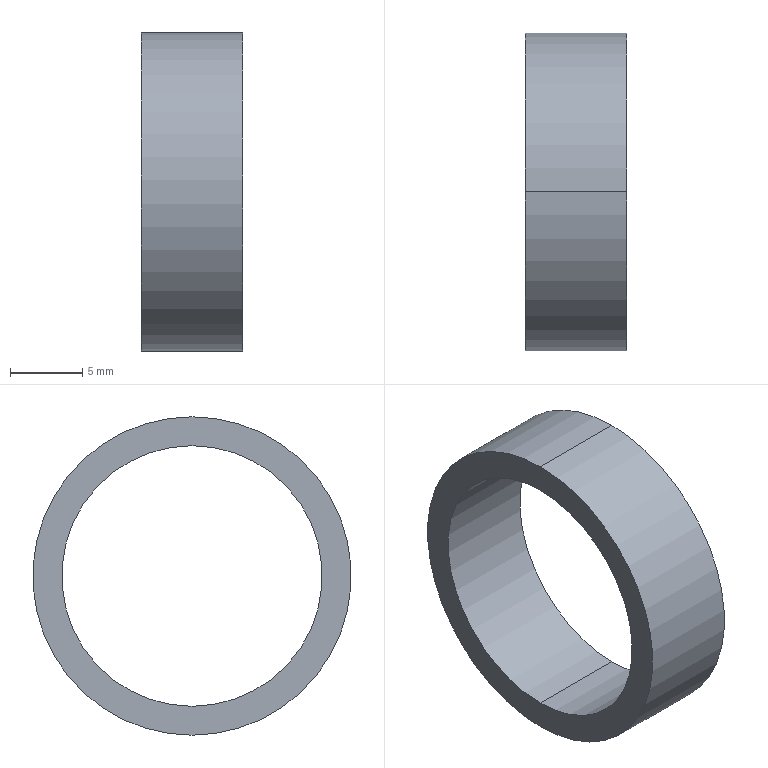Part | SolidWorks | features BaseBody 1 | 1 solid | 6 faces | box 7 x 22 x 22 mm | volume 879.646 mm3 | cylinder 4 | plane 2 | commonest cylinder face diameters 18 x2 22 x2
STEP:
#1=CARTESIAN_POINT('',(-3.5,0.,-11.));
#2=VERTEX_POINT('',#1);
#3=CARTESIAN_POINT('',(-3.5,0.,11.));
#4=VERTEX_POINT('',#3);
#5=CARTESIAN_POINT('',(-3.5,0.,0.));
#6=DIRECTION('',(1.,0.,0.));
#7=DIRECTION('',(0.,0.,-1.));
#8=AXIS2_PLACEMENT_3D('',#5,#6,#7);
#9=CIRCLE('',#8,11.);
#10=EDGE_CURVE('',#2,#4,#9,.T.);
#11=ORIENTED_EDGE('',*,*,#10,.T.);
#12=CARTESIAN_POINT('',(3.5,0.,11.));
#13=VERTEX_POINT('',#12);
#14=CARTESIAN_POINT('',(-3.5,0.,11.));
#15=DIRECTION('',(1.,0.,0.));
#16=VECTOR('',#15,1000.);
#17=LINE('',#14,#16);
#18=EDGE_CURVE('',#4,#13,#17,.T.);
#19=ORIENTED_EDGE('',*,*,#18,.T.);
#20=CARTESIAN_POINT('',(3.5,0.,-11.));
#21=VERTEX_POINT('',#20);
#22=CARTESIAN_POINT('',(3.5,0.,0.));
#23=DIRECTION('',(-1.,0.,0.));
#24=DIRECTION('',(0.,0.,-1.));
#25=AXIS2_PLACEMENT_3D('',#22,#23,#24);
#26=CIRCLE('',#25,11.);
#27=EDGE_CURVE('',#13,#21,#26,.T.);
#28=ORIENTED_EDGE('',*,*,#27,.T.);
#29=CARTESIAN_POINT('',(-3.5,0.,-11.));
#30=DIRECTION('',(1.,0.,0.));
#31=VECTOR('',#30,1000.);
#32=LINE('',#29,#31);
#33=EDGE_CURVE('',#2,#21,#32,.T.);
#34=ORIENTED_EDGE('',*,*,#33,.F.);
#35=EDGE_LOOP('',(#11,#19,#28,#34));
#36=FACE_OUTER_BOUND('',#35,.T.);
#37=CARTESIAN_POINT('',(-3.5,0.,0.));
#38=DIRECTION('',(1.,0.,0.));
#39=DIRECTION('',(0.,0.,-1.));
#40=AXIS2_PLACEMENT_3D('',#37,#38,#39);
#41=CYLINDRICAL_SURFACE('',#40,11.);
#42=ADVANCED_FACE('',(#36),#41,.T.);
#43=CARTESIAN_POINT('',(-3.5,0.,-9.));
#44=VERTEX_POINT('',#43);
#45=CARTESIAN_POINT('',(-3.5,0.,9.));
#46=VERTEX_POINT('',#45);
#47=CARTESIAN_POINT('',(-3.5,0.,0.));
#48=DIRECTION('',(-1.,0.,0.));
#49=DIRECTION('',(0.,0.,-1.));
#50=AXIS2_PLACEMENT_3D('',#47,#48,#49);
#51=CIRCLE('',#50,9.);
#52=EDGE_CURVE('',#44,#46,#51,.T.);
#53=ORIENTED_EDGE('',*,*,#52,.T.);
#54=CARTESIAN_POINT('',(3.5,0.,9.));
#55=VERTEX_POINT('',#54);
#56=CARTESIAN_POINT('',(-4.5,0.,9.));
#57=DIRECTION('',(1.,0.,0.));
#58=VECTOR('',#57,1000.);
#59=LINE('',#56,#58);
#60=EDGE_CURVE('',#46,#55,#59,.T.);
#61=ORIENTED_EDGE('',*,*,#60,.T.);
#62=CARTESIAN_POINT('',(3.5,0.,-9.));
#63=VERTEX_POINT('',#62);
#64=CARTESIAN_POINT('',(3.5,0.,0.));
#65=DIRECTION('',(-1.,0.,0.));
#66=DIRECTION('',(0.,0.,-1.));
#67=AXIS2_PLACEMENT_3D('',#64,#65,#66);
#68=CIRCLE('',#67,9.);
#69=EDGE_CURVE('',#63,#55,#68,.T.);
#70=ORIENTED_EDGE('',*,*,#69,.F.);
#71=CARTESIAN_POINT('',(-4.5,0.,-9.));
#72=DIRECTION('',(1.,0.,0.));
#73=VECTOR('',#72,1000.);
#74=LINE('',#71,#73);
#75=EDGE_CURVE('',#44,#63,#74,.T.);
#76=ORIENTED_EDGE('',*,*,#75,.F.);
#77=EDGE_LOOP('',(#53,#61,#70,#76));
#78=FACE_OUTER_BOUND('',#77,.T.);
#79=CARTESIAN_POINT('',(-4.5,0.,0.));
#80=DIRECTION('',(1.,0.,0.));
#81=DIRECTION('',(0.,0.,-1.));
#82=AXIS2_PLACEMENT_3D('',#79,#80,#81);
#83=CYLINDRICAL_SURFACE('',#82,9.);
#84=ADVANCED_FACE('',(#78),#83,.F.);
#85=ORIENTED_EDGE('',*,*,#18,.F.);
#86=CARTESIAN_POINT('',(-3.5,0.,0.));
#87=DIRECTION('',(1.,0.,0.));
#88=DIRECTION('',(0.,0.,-1.));
#89=AXIS2_PLACEMENT_3D('',#86,#87,#88);
#90=CIRCLE('',#89,11.);
#91=EDGE_CURVE('',#4,#2,#90,.T.);
#92=ORIENTED_EDGE('',*,*,#91,.T.);
#93=ORIENTED_EDGE('',*,*,#33,.T.);
#94=CARTESIAN_POINT('',(3.5,0.,0.));
#95=DIRECTION('',(-1.,0.,0.));
#96=DIRECTION('',(0.,0.,-1.));
#97=AXIS2_PLACEMENT_3D('',#94,#95,#96);
#98=CIRCLE('',#97,11.);
#99=EDGE_CURVE('',#21,#13,#98,.T.);
#100=ORIENTED_EDGE('',*,*,#99,.T.);
#101=EDGE_LOOP('',(#85,#92,#93,#100));
#102=FACE_OUTER_BOUND('',#101,.T.);
#103=CARTESIAN_POINT('',(-3.5,0.,0.));
#104=DIRECTION('',(1.,0.,0.));
#105=DIRECTION('',(0.,0.,-1.));
#106=AXIS2_PLACEMENT_3D('',#103,#104,#105);
#107=CYLINDRICAL_SURFACE('',#106,11.);
#108=ADVANCED_FACE('',(#102),#107,.T.);
#109=ORIENTED_EDGE('',*,*,#52,.F.);
#110=CARTESIAN_POINT('',(-3.5,0.,0.));
#111=DIRECTION('',(-1.,0.,0.));
#112=DIRECTION('',(0.,0.,-1.));
#113=AXIS2_PLACEMENT_3D('',#110,#111,#112);
#114=CIRCLE('',#113,9.);
#115=EDGE_CURVE('',#46,#44,#114,.T.);
#116=ORIENTED_EDGE('',*,*,#115,.F.);
#117=EDGE_LOOP('',(#109,#116));
#118=FACE_BOUND('',#117,.T.);
#119=ORIENTED_EDGE('',*,*,#10,.F.);
#120=ORIENTED_EDGE('',*,*,#91,.F.);
#121=EDGE_LOOP('',(#119,#120));
#122=FACE_OUTER_BOUND('',#121,.T.);
#123=CARTESIAN_POINT('',(-3.5,0.,0.));
#124=DIRECTION('',(1.,0.,0.));
#125=DIRECTION('',(0.,0.,-1.));
#126=AXIS2_PLACEMENT_3D('',#123,#124,#125);
#127=PLANE('',#126);
#128=ADVANCED_FACE('',(#118,#122),#127,.F.);
#129=ORIENTED_EDGE('',*,*,#69,.T.);
#130=CARTESIAN_POINT('',(3.5,0.,0.));
#131=DIRECTION('',(-1.,0.,0.));
#132=DIRECTION('',(0.,0.,-1.));
#133=AXIS2_PLACEMENT_3D('',#130,#131,#132);
#134=CIRCLE('',#133,9.);
#135=EDGE_CURVE('',#55,#63,#134,.T.);
#136=ORIENTED_EDGE('',*,*,#135,.T.);
#137=EDGE_LOOP('',(#129,#136));
#138=FACE_BOUND('',#137,.T.);
#139=ORIENTED_EDGE('',*,*,#99,.F.);
#140=ORIENTED_EDGE('',*,*,#27,.F.);
#141=EDGE_LOOP('',(#139,#140));
#142=FACE_OUTER_BOUND('',#141,.T.);
#143=CARTESIAN_POINT('',(3.5,0.,0.));
#144=DIRECTION('',(1.,0.,0.));
#145=DIRECTION('',(0.,0.,-1.));
#146=AXIS2_PLACEMENT_3D('',#143,#144,#145);
#147=PLANE('',#146);
#148=ADVANCED_FACE('',(#138,#142),#147,.T.);
#149=ORIENTED_EDGE('',*,*,#60,.F.);
#150=ORIENTED_EDGE('',*,*,#115,.T.);
#151=ORIENTED_EDGE('',*,*,#75,.T.);
#152=ORIENTED_EDGE('',*,*,#135,.F.);
#153=EDGE_LOOP('',(#149,#150,#151,#152));
#154=FACE_OUTER_BOUND('',#153,.T.);
#155=CARTESIAN_POINT('',(-4.5,0.,0.));
#156=DIRECTION('',(1.,0.,0.));
#157=DIRECTION('',(0.,0.,-1.));
#158=AXIS2_PLACEMENT_3D('',#155,#156,#157);
#159=CYLINDRICAL_SURFACE('',#158,9.);
#160=ADVANCED_FACE('',(#154),#159,.F.);
#161=CLOSED_SHELL('',(#42,#84,#108,#128,#148,#160));
#162=MANIFOLD_SOLID_BREP('',#161);
#163=CARTESIAN_POINT('',(0.,0.,0.));
#164=DIRECTION('',(0.,0.,1.));
#165=DIRECTION('',(1.,0.,0.));
#166=AXIS2_PLACEMENT_3D('',#163,#164,#165);
#167=(LENGTH_UNIT()NAMED_UNIT(*)SI_UNIT(.MILLI.,.METRE.));
#168=UNCERTAINTY_MEASURE_WITH_UNIT(LENGTH_MEASURE(0.00001),#167,'','');
#169=(NAMED_UNIT(*)PLANE_ANGLE_UNIT()SI_UNIT($,.RADIAN.));
#170=(NAMED_UNIT(*)SI_UNIT($,.STERADIAN.)SOLID_ANGLE_UNIT());
#171=(GEOMETRIC_REPRESENTATION_CONTEXT(3)GLOBAL_UNCERTAINTY_ASSIGNED_CONTEXT((#168))GLOBAL_UNIT_ASSIGNED_CONTEXT((#167,#169,#170))REPRESENTATION_CONTEXT('',''));
#172=ADVANCED_BREP_SHAPE_REPRESENTATION('',(#162,#166),#171);